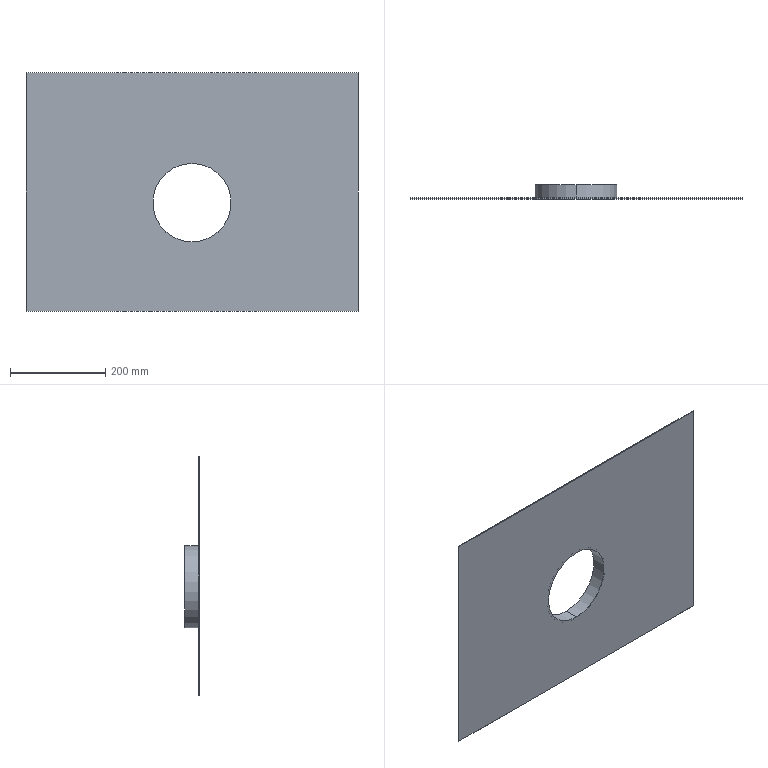Part | SolidWorks | features ICE 2, FlatPattern 1, SMBaseFlange 1, SheetMetal 1 | 1 solid | 11 faces | box 698 x 30 x 501 mm | volume 716095 mm3 | plane 7 | cylinder 4 | commonest cylinder face diameters 165 x2 173 x2
STEP:
#1=CARTESIAN_POINT('',(0.,28.,-105.));
#2=VERTEX_POINT('',#1);
#3=CARTESIAN_POINT('',(0.,28.,60.));
#4=VERTEX_POINT('',#3);
#5=CARTESIAN_POINT('',(0.,28.,-22.5));
#6=DIRECTION('',(0.,1.,0.));
#7=DIRECTION('',(0.,0.,1.));
#8=AXIS2_PLACEMENT_3D('',#5,#6,#7);
#9=CIRCLE('',#8,82.5);
#10=EDGE_CURVE('',#2,#4,#9,.T.);
#11=ORIENTED_EDGE('',*,*,#10,.T.);
#12=CARTESIAN_POINT('',(0.,-2.,60.));
#13=VERTEX_POINT('',#12);
#14=CARTESIAN_POINT('',(0.,28.,60.));
#15=DIRECTION('',(0.,-1.,0.));
#16=VECTOR('',#15,1000.);
#17=LINE('',#14,#16);
#18=EDGE_CURVE('',#4,#13,#17,.T.);
#19=ORIENTED_EDGE('',*,*,#18,.T.);
#20=CARTESIAN_POINT('',(0.,-2.,-105.));
#21=VERTEX_POINT('',#20);
#22=CARTESIAN_POINT('',(0.,-2.,-22.5));
#23=DIRECTION('',(0.,1.,0.));
#24=DIRECTION('',(0.,0.,1.));
#25=AXIS2_PLACEMENT_3D('',#22,#23,#24);
#26=CIRCLE('',#25,82.5);
#27=EDGE_CURVE('',#21,#13,#26,.T.);
#28=ORIENTED_EDGE('',*,*,#27,.F.);
#29=CARTESIAN_POINT('',(0.,28.,-105.));
#30=DIRECTION('',(0.,-1.,0.));
#31=VECTOR('',#30,1000.);
#32=LINE('',#29,#31);
#33=EDGE_CURVE('',#2,#21,#32,.T.);
#34=ORIENTED_EDGE('',*,*,#33,.F.);
#35=EDGE_LOOP('',(#11,#19,#28,#34));
#36=FACE_OUTER_BOUND('',#35,.T.);
#37=CARTESIAN_POINT('',(0.,28.,-22.5));
#38=DIRECTION('',(0.,-1.,0.));
#39=DIRECTION('',(0.,0.,-1.));
#40=AXIS2_PLACEMENT_3D('',#37,#38,#39);
#41=CYLINDRICAL_SURFACE('',#40,82.5);
#42=ADVANCED_FACE('',(#36),#41,.F.);
#43=CARTESIAN_POINT('',(0.,28.,64.));
#44=VERTEX_POINT('',#43);
#45=CARTESIAN_POINT('',(0.,28.,-109.));
#46=VERTEX_POINT('',#45);
#47=CARTESIAN_POINT('',(0.,28.,-22.5));
#48=DIRECTION('',(0.,1.,0.));
#49=DIRECTION('',(0.,0.,1.));
#50=AXIS2_PLACEMENT_3D('',#47,#48,#49);
#51=CIRCLE('',#50,86.5);
#52=EDGE_CURVE('',#44,#46,#51,.T.);
#53=ORIENTED_EDGE('',*,*,#52,.F.);
#54=CARTESIAN_POINT('',(0.,0.,64.));
#55=VERTEX_POINT('',#54);
#56=CARTESIAN_POINT('',(0.,28.,64.));
#57=DIRECTION('',(0.,-1.,0.));
#58=VECTOR('',#57,1000.);
#59=LINE('',#56,#58);
#60=EDGE_CURVE('',#44,#55,#59,.T.);
#61=ORIENTED_EDGE('',*,*,#60,.T.);
#62=CARTESIAN_POINT('',(0.,0.,-109.));
#63=VERTEX_POINT('',#62);
#64=CARTESIAN_POINT('',(0.,0.,-22.5));
#65=DIRECTION('',(0.,1.,0.));
#66=DIRECTION('',(0.,0.,1.));
#67=AXIS2_PLACEMENT_3D('',#64,#65,#66);
#68=CIRCLE('',#67,86.5);
#69=EDGE_CURVE('',#55,#63,#68,.T.);
#70=ORIENTED_EDGE('',*,*,#69,.T.);
#71=CARTESIAN_POINT('',(0.,28.,-109.));
#72=DIRECTION('',(0.,-1.,0.));
#73=VECTOR('',#72,1000.);
#74=LINE('',#71,#73);
#75=EDGE_CURVE('',#46,#63,#74,.T.);
#76=ORIENTED_EDGE('',*,*,#75,.F.);
#77=EDGE_LOOP('',(#53,#61,#70,#76));
#78=FACE_OUTER_BOUND('',#77,.T.);
#79=CARTESIAN_POINT('',(0.,28.,-22.5));
#80=DIRECTION('',(0.,-1.,0.));
#81=DIRECTION('',(0.,0.,-1.));
#82=AXIS2_PLACEMENT_3D('',#79,#80,#81);
#83=CYLINDRICAL_SURFACE('',#82,86.5);
#84=ADVANCED_FACE('',(#78),#83,.T.);
#85=CARTESIAN_POINT('',(349.,0.,250.5));
#86=VERTEX_POINT('',#85);
#87=CARTESIAN_POINT('',(349.,0.,-250.5));
#88=VERTEX_POINT('',#87);
#89=CARTESIAN_POINT('',(349.,0.,-250.5));
#90=DIRECTION('',(0.,0.,-1.));
#91=VECTOR('',#90,1000.);
#92=LINE('',#89,#91);
#93=EDGE_CURVE('',#86,#88,#92,.T.);
#94=ORIENTED_EDGE('',*,*,#93,.F.);
#95=CARTESIAN_POINT('',(349.,-2.,250.5));
#96=VERTEX_POINT('',#95);
#97=CARTESIAN_POINT('',(349.,-2.,250.5));
#98=DIRECTION('',(0.,1.,0.));
#99=VECTOR('',#98,1000.);
#100=LINE('',#97,#99);
#101=EDGE_CURVE('',#96,#86,#100,.T.);
#102=ORIENTED_EDGE('',*,*,#101,.F.);
#103=CARTESIAN_POINT('',(349.,-2.,-250.5));
#104=VERTEX_POINT('',#103);
#105=CARTESIAN_POINT('',(349.,-2.,-250.5));
#106=DIRECTION('',(0.,0.,-1.));
#107=VECTOR('',#106,1000.);
#108=LINE('',#105,#107);
#109=EDGE_CURVE('',#96,#104,#108,.T.);
#110=ORIENTED_EDGE('',*,*,#109,.T.);
#111=CARTESIAN_POINT('',(349.,-2.,-250.5));
#112=DIRECTION('',(0.,1.,0.));
#113=VECTOR('',#112,1000.);
#114=LINE('',#111,#113);
#115=EDGE_CURVE('',#104,#88,#114,.T.);
#116=ORIENTED_EDGE('',*,*,#115,.T.);
#117=EDGE_LOOP('',(#94,#102,#110,#116));
#118=FACE_OUTER_BOUND('',#117,.T.);
#119=CARTESIAN_POINT('',(349.,-2.,-250.5));
#120=DIRECTION('',(1.,0.,0.));
#121=DIRECTION('',(0.,0.,-1.));
#122=AXIS2_PLACEMENT_3D('',#119,#120,#121);
#123=PLANE('',#122);
#124=ADVANCED_FACE('',(#118),#123,.T.);
#125=CARTESIAN_POINT('',(-349.,0.,250.5));
#126=VERTEX_POINT('',#125);
#127=CARTESIAN_POINT('',(-349.,0.,250.5));
#128=DIRECTION('',(1.,0.,0.));
#129=VECTOR('',#128,1000.);
#130=LINE('',#127,#129);
#131=EDGE_CURVE('',#126,#86,#130,.T.);
#132=ORIENTED_EDGE('',*,*,#131,.F.);
#133=CARTESIAN_POINT('',(-349.,-2.,250.5));
#134=VERTEX_POINT('',#133);
#135=CARTESIAN_POINT('',(-349.,-2.,250.5));
#136=DIRECTION('',(0.,1.,0.));
#137=VECTOR('',#136,1000.);
#138=LINE('',#135,#137);
#139=EDGE_CURVE('',#134,#126,#138,.T.);
#140=ORIENTED_EDGE('',*,*,#139,.F.);
#141=CARTESIAN_POINT('',(-349.,-2.,250.5));
#142=DIRECTION('',(1.,0.,0.));
#143=VECTOR('',#142,1000.);
#144=LINE('',#141,#143);
#145=EDGE_CURVE('',#134,#96,#144,.T.);
#146=ORIENTED_EDGE('',*,*,#145,.T.);
#147=ORIENTED_EDGE('',*,*,#101,.T.);
#148=EDGE_LOOP('',(#132,#140,#146,#147));
#149=FACE_OUTER_BOUND('',#148,.T.);
#150=CARTESIAN_POINT('',(-349.,-2.,250.5));
#151=DIRECTION('',(0.,0.,1.));
#152=DIRECTION('',(1.,0.,0.));
#153=AXIS2_PLACEMENT_3D('',#150,#151,#152);
#154=PLANE('',#153);
#155=ADVANCED_FACE('',(#149),#154,.T.);
#156=CARTESIAN_POINT('',(-349.,0.,-250.5));
#157=VERTEX_POINT('',#156);
#158=CARTESIAN_POINT('',(-349.,0.,-250.5));
#159=DIRECTION('',(0.,0.,1.));
#160=VECTOR('',#159,1000.);
#161=LINE('',#158,#160);
#162=EDGE_CURVE('',#157,#126,#161,.T.);
#163=ORIENTED_EDGE('',*,*,#162,.F.);
#164=CARTESIAN_POINT('',(-349.,-2.,-250.5));
#165=VERTEX_POINT('',#164);
#166=CARTESIAN_POINT('',(-349.,-2.,-250.5));
#167=DIRECTION('',(0.,1.,0.));
#168=VECTOR('',#167,1000.);
#169=LINE('',#166,#168);
#170=EDGE_CURVE('',#165,#157,#169,.T.);
#171=ORIENTED_EDGE('',*,*,#170,.F.);
#172=CARTESIAN_POINT('',(-349.,-2.,-250.5));
#173=DIRECTION('',(0.,0.,1.));
#174=VECTOR('',#173,1000.);
#175=LINE('',#172,#174);
#176=EDGE_CURVE('',#165,#134,#175,.T.);
#177=ORIENTED_EDGE('',*,*,#176,.T.);
#178=ORIENTED_EDGE('',*,*,#139,.T.);
#179=EDGE_LOOP('',(#163,#171,#177,#178));
#180=FACE_OUTER_BOUND('',#179,.T.);
#181=CARTESIAN_POINT('',(-349.,-2.,-250.5));
#182=DIRECTION('',(-1.,0.,0.));
#183=DIRECTION('',(0.,0.,1.));
#184=AXIS2_PLACEMENT_3D('',#181,#182,#183);
#185=PLANE('',#184);
#186=ADVANCED_FACE('',(#180),#185,.T.);
#187=CARTESIAN_POINT('',(-349.,0.,-250.5));
#188=DIRECTION('',(-1.,0.,0.));
#189=VECTOR('',#188,1000.);
#190=LINE('',#187,#189);
#191=EDGE_CURVE('',#88,#157,#190,.T.);
#192=ORIENTED_EDGE('',*,*,#191,.F.);
#193=ORIENTED_EDGE('',*,*,#115,.F.);
#194=CARTESIAN_POINT('',(-349.,-2.,-250.5));
#195=DIRECTION('',(-1.,0.,0.));
#196=VECTOR('',#195,1000.);
#197=LINE('',#194,#196);
#198=EDGE_CURVE('',#104,#165,#197,.T.);
#199=ORIENTED_EDGE('',*,*,#198,.T.);
#200=ORIENTED_EDGE('',*,*,#170,.T.);
#201=EDGE_LOOP('',(#192,#193,#199,#200));
#202=FACE_OUTER_BOUND('',#201,.T.);
#203=CARTESIAN_POINT('',(-349.,-2.,-250.5));
#204=DIRECTION('',(0.,0.,-1.));
#205=DIRECTION('',(-1.,0.,0.));
#206=AXIS2_PLACEMENT_3D('',#203,#204,#205);
#207=PLANE('',#206);
#208=ADVANCED_FACE('',(#202),#207,.T.);
#209=ORIENTED_EDGE('',*,*,#109,.F.);
#210=ORIENTED_EDGE('',*,*,#145,.F.);
#211=ORIENTED_EDGE('',*,*,#176,.F.);
#212=ORIENTED_EDGE('',*,*,#198,.F.);
#213=EDGE_LOOP('',(#209,#210,#211,#212));
#214=FACE_OUTER_BOUND('',#213,.T.);
#215=ORIENTED_EDGE('',*,*,#27,.T.);
#216=CARTESIAN_POINT('',(0.,-2.,-22.5));
#217=DIRECTION('',(0.,1.,0.));
#218=DIRECTION('',(0.,0.,1.));
#219=AXIS2_PLACEMENT_3D('',#216,#217,#218);
#220=CIRCLE('',#219,82.5);
#221=EDGE_CURVE('',#13,#21,#220,.T.);
#222=ORIENTED_EDGE('',*,*,#221,.T.);
#223=EDGE_LOOP('',(#215,#222));
#224=FACE_BOUND('',#223,.T.);
#225=CARTESIAN_POINT('',(0.,-2.,0.));
#226=DIRECTION('',(0.,1.,0.));
#227=DIRECTION('',(0.,0.,1.));
#228=AXIS2_PLACEMENT_3D('',#225,#226,#227);
#229=PLANE('',#228);
#230=ADVANCED_FACE('',(#214,#224),#229,.F.);
#231=CARTESIAN_POINT('',(0.,0.,-22.5));
#232=DIRECTION('',(0.,1.,0.));
#233=DIRECTION('',(0.,0.,1.));
#234=AXIS2_PLACEMENT_3D('',#231,#232,#233);
#235=CIRCLE('',#234,86.5);
#236=EDGE_CURVE('',#63,#55,#235,.T.);
#237=ORIENTED_EDGE('',*,*,#236,.F.);
#238=ORIENTED_EDGE('',*,*,#69,.F.);
#239=EDGE_LOOP('',(#237,#238));
#240=FACE_BOUND('',#239,.T.);
#241=ORIENTED_EDGE('',*,*,#93,.T.);
#242=ORIENTED_EDGE('',*,*,#191,.T.);
#243=ORIENTED_EDGE('',*,*,#162,.T.);
#244=ORIENTED_EDGE('',*,*,#131,.T.);
#245=EDGE_LOOP('',(#241,#242,#243,#244));
#246=FACE_OUTER_BOUND('',#245,.T.);
#247=CARTESIAN_POINT('',(0.,0.,0.));
#248=DIRECTION('',(0.,1.,0.));
#249=DIRECTION('',(0.,0.,1.));
#250=AXIS2_PLACEMENT_3D('',#247,#248,#249);
#251=PLANE('',#250);
#252=ADVANCED_FACE('',(#240,#246),#251,.T.);
#253=CARTESIAN_POINT('',(0.,28.,-22.5));
#254=DIRECTION('',(0.,1.,0.));
#255=DIRECTION('',(0.,0.,1.));
#256=AXIS2_PLACEMENT_3D('',#253,#254,#255);
#257=CIRCLE('',#256,86.5);
#258=EDGE_CURVE('',#46,#44,#257,.T.);
#259=ORIENTED_EDGE('',*,*,#258,.T.);
#260=ORIENTED_EDGE('',*,*,#52,.T.);
#261=EDGE_LOOP('',(#259,#260));
#262=FACE_OUTER_BOUND('',#261,.T.);
#263=ORIENTED_EDGE('',*,*,#10,.F.);
#264=CARTESIAN_POINT('',(0.,28.,-22.5));
#265=DIRECTION('',(0.,1.,0.));
#266=DIRECTION('',(0.,0.,1.));
#267=AXIS2_PLACEMENT_3D('',#264,#265,#266);
#268=CIRCLE('',#267,82.5);
#269=EDGE_CURVE('',#4,#2,#268,.T.);
#270=ORIENTED_EDGE('',*,*,#269,.F.);
#271=EDGE_LOOP('',(#263,#270));
#272=FACE_BOUND('',#271,.T.);
#273=CARTESIAN_POINT('',(0.,28.,-22.5));
#274=DIRECTION('',(0.,1.,0.));
#275=DIRECTION('',(0.,0.,1.));
#276=AXIS2_PLACEMENT_3D('',#273,#274,#275);
#277=PLANE('',#276);
#278=ADVANCED_FACE('',(#262,#272),#277,.T.);
#279=ORIENTED_EDGE('',*,*,#60,.F.);
#280=ORIENTED_EDGE('',*,*,#258,.F.);
#281=ORIENTED_EDGE('',*,*,#75,.T.);
#282=ORIENTED_EDGE('',*,*,#236,.T.);
#283=EDGE_LOOP('',(#279,#280,#281,#282));
#284=FACE_OUTER_BOUND('',#283,.T.);
#285=CARTESIAN_POINT('',(0.,28.,-22.5));
#286=DIRECTION('',(0.,-1.,0.));
#287=DIRECTION('',(0.,0.,-1.));
#288=AXIS2_PLACEMENT_3D('',#285,#286,#287);
#289=CYLINDRICAL_SURFACE('',#288,86.5);
#290=ADVANCED_FACE('',(#284),#289,.T.);
#291=ORIENTED_EDGE('',*,*,#18,.F.);
#292=ORIENTED_EDGE('',*,*,#269,.T.);
#293=ORIENTED_EDGE('',*,*,#33,.T.);
#294=ORIENTED_EDGE('',*,*,#221,.F.);
#295=EDGE_LOOP('',(#291,#292,#293,#294));
#296=FACE_OUTER_BOUND('',#295,.T.);
#297=CARTESIAN_POINT('',(0.,28.,-22.5));
#298=DIRECTION('',(0.,-1.,0.));
#299=DIRECTION('',(0.,0.,-1.));
#300=AXIS2_PLACEMENT_3D('',#297,#298,#299);
#301=CYLINDRICAL_SURFACE('',#300,82.5);
#302=ADVANCED_FACE('',(#296),#301,.F.);
#303=CLOSED_SHELL('',(#42,#84,#124,#155,#186,#208,#230,#252,#278,#290,#302));
#304=MANIFOLD_SOLID_BREP('',#303);
#305=CARTESIAN_POINT('',(0.,0.,0.));
#306=DIRECTION('',(0.,0.,1.));
#307=DIRECTION('',(1.,0.,0.));
#308=AXIS2_PLACEMENT_3D('',#305,#306,#307);
#309=(LENGTH_UNIT()NAMED_UNIT(*)SI_UNIT(.MILLI.,.METRE.));
#310=UNCERTAINTY_MEASURE_WITH_UNIT(LENGTH_MEASURE(0.00001),#309,'','');
#311=(NAMED_UNIT(*)PLANE_ANGLE_UNIT()SI_UNIT($,.RADIAN.));
#312=(NAMED_UNIT(*)SI_UNIT($,.STERADIAN.)SOLID_ANGLE_UNIT());
#313=(GEOMETRIC_REPRESENTATION_CONTEXT(3)GLOBAL_UNCERTAINTY_ASSIGNED_CONTEXT((#310))GLOBAL_UNIT_ASSIGNED_CONTEXT((#309,#311,#312))REPRESENTATION_CONTEXT('',''));
#314=ADVANCED_BREP_SHAPE_REPRESENTATION('',(#304,#308),#313);